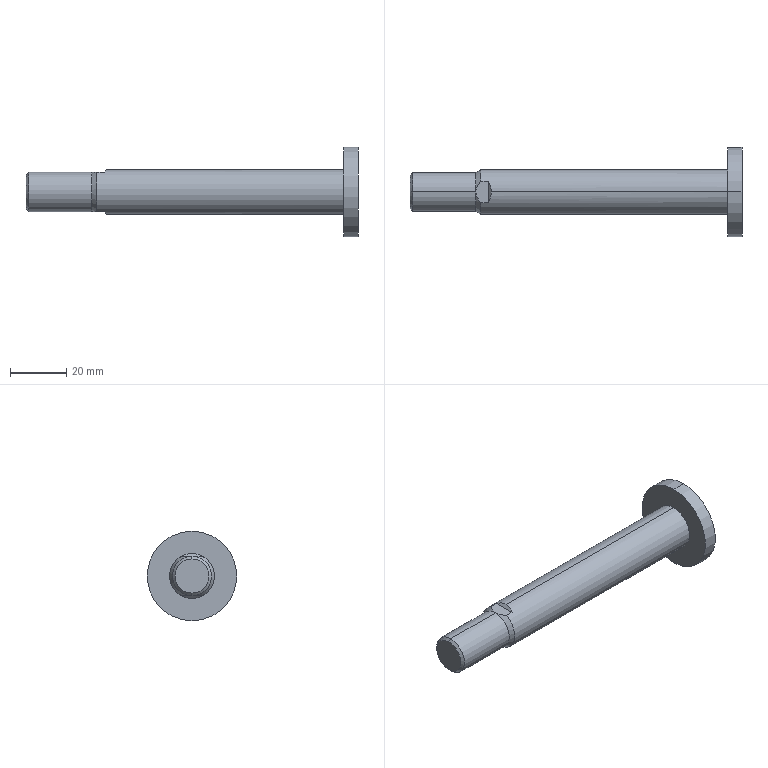Part | SolidWorks | features BaseBody 1 | 1 solid | 17 faces | box 118.5 x 32 x 32 mm | volume 25635 mm3 | plane 7 | cylinder 6 | cone 4 | commonest cylinder face diameters 14 x2 16 x2 32 x2
STEP:
#1=CARTESIAN_POINT('',(-0.5,3.873,7.));
#2=VERTEX_POINT('',#1);
#3=CARTESIAN_POINT('',(0.5,0.,8.));
#4=VERTEX_POINT('',#3);
#5=CARTESIAN_POINT('',(-0.5,3.873,7.));
#6=CARTESIAN_POINT('',(0.1595,2.681,7.659));
#7=CARTESIAN_POINT('',(0.5,1.362,8.));
#8=CARTESIAN_POINT('',(0.5,0.,8.));
#9=(BOUNDED_CURVE()B_SPLINE_CURVE(3,(#5,#6,#7,#8),.UNSPECIFIED.,.F.,.F.)B_SPLINE_CURVE_WITH_KNOTS((4,4),(5.778,6.283),.UNSPECIFIED.)CURVE()GEOMETRIC_REPRESENTATION_ITEM()RATIONAL_B_SPLINE_CURVE((1.,0.9788,0.9788,1.))REPRESENTATION_ITEM(''));
#10=EDGE_CURVE('',#2,#4,#9,.T.);
#11=ORIENTED_EDGE('',*,*,#10,.T.);
#12=CARTESIAN_POINT('',(85.,0.,8.));
#13=VERTEX_POINT('',#12);
#14=CARTESIAN_POINT('',(90.,0.,8.));
#15=DIRECTION('',(1.,0.,0.));
#16=VECTOR('',#15,1000.);
#17=LINE('',#14,#16);
#18=EDGE_CURVE('',#4,#13,#17,.T.);
#19=ORIENTED_EDGE('',*,*,#18,.T.);
#20=CARTESIAN_POINT('',(85.,0.,-8.));
#21=VERTEX_POINT('',#20);
#22=CARTESIAN_POINT('',(85.,0.,0.));
#23=DIRECTION('',(-1.,0.,0.));
#24=DIRECTION('',(0.,0.,-1.));
#25=AXIS2_PLACEMENT_3D('',#22,#23,#24);
#26=CIRCLE('',#25,8.);
#27=EDGE_CURVE('',#13,#21,#26,.T.);
#28=ORIENTED_EDGE('',*,*,#27,.T.);
#29=CARTESIAN_POINT('',(0.5,0.,-8.));
#30=VERTEX_POINT('',#29);
#31=CARTESIAN_POINT('',(90.,0.,-8.));
#32=DIRECTION('',(1.,0.,0.));
#33=VECTOR('',#32,1000.);
#34=LINE('',#31,#33);
#35=EDGE_CURVE('',#30,#21,#34,.T.);
#36=ORIENTED_EDGE('',*,*,#35,.F.);
#37=CARTESIAN_POINT('',(-0.5,3.873,-7.));
#38=VERTEX_POINT('',#37);
#39=CARTESIAN_POINT('',(0.5,0.,-8.));
#40=CARTESIAN_POINT('',(0.5,1.362,-8.));
#41=CARTESIAN_POINT('',(0.1595,2.681,-7.659));
#42=CARTESIAN_POINT('',(-0.5,3.873,-7.));
#43=(BOUNDED_CURVE()B_SPLINE_CURVE(3,(#39,#40,#41,#42),.UNSPECIFIED.,.F.,.F.)B_SPLINE_CURVE_WITH_KNOTS((4,4),(0.,0.5054),.UNSPECIFIED.)CURVE()GEOMETRIC_REPRESENTATION_ITEM()RATIONAL_B_SPLINE_CURVE((1.,0.9788,0.9788,1.))REPRESENTATION_ITEM(''));
#44=EDGE_CURVE('',#30,#38,#43,.T.);
#45=ORIENTED_EDGE('',*,*,#44,.T.);
#46=CARTESIAN_POINT('',(-3.268,3.873,-7.));
#47=VERTEX_POINT('',#46);
#48=CARTESIAN_POINT('',(90.,3.873,-7.));
#49=DIRECTION('',(-1.,0.,0.));
#50=VECTOR('',#49,1000.);
#51=LINE('',#48,#50);
#52=EDGE_CURVE('',#38,#47,#51,.T.);
#53=ORIENTED_EDGE('',*,*,#52,.T.);
#54=CARTESIAN_POINT('',(-3.268,3.873,7.));
#55=VERTEX_POINT('',#54);
#56=CARTESIAN_POINT('',(-3.268,0.,0.));
#57=DIRECTION('',(1.,0.,0.));
#58=DIRECTION('',(0.,0.,-1.));
#59=AXIS2_PLACEMENT_3D('',#56,#57,#58);
#60=CIRCLE('',#59,8.);
#61=EDGE_CURVE('',#47,#55,#60,.T.);
#62=ORIENTED_EDGE('',*,*,#61,.T.);
#63=CARTESIAN_POINT('',(90.,3.873,7.));
#64=DIRECTION('',(1.,0.,0.));
#65=VECTOR('',#64,1000.);
#66=LINE('',#63,#65);
#67=EDGE_CURVE('',#55,#2,#66,.T.);
#68=ORIENTED_EDGE('',*,*,#67,.T.);
#69=EDGE_LOOP('',(#11,#19,#28,#36,#45,#53,#62,#68));
#70=FACE_OUTER_BOUND('',#69,.T.);
#71=CARTESIAN_POINT('',(90.,0.,0.));
#72=DIRECTION('',(1.,0.,0.));
#73=DIRECTION('',(0.,0.,-1.));
#74=AXIS2_PLACEMENT_3D('',#71,#72,#73);
#75=CYLINDRICAL_SURFACE('',#74,8.);
#76=ADVANCED_FACE('',(#70),#75,.T.);
#77=CARTESIAN_POINT('',(-27.58,0.,-7.));
#78=VERTEX_POINT('',#77);
#79=CARTESIAN_POINT('',(-27.58,0.,7.));
#80=VERTEX_POINT('',#79);
#81=CARTESIAN_POINT('',(-27.58,0.,0.));
#82=DIRECTION('',(1.,0.,0.));
#83=DIRECTION('',(0.,0.,-1.));
#84=AXIS2_PLACEMENT_3D('',#81,#82,#83);
#85=CIRCLE('',#84,7.);
#86=EDGE_CURVE('',#78,#80,#85,.T.);
#87=ORIENTED_EDGE('',*,*,#86,.T.);
#88=CARTESIAN_POINT('',(-5.,0.,7.));
#89=VERTEX_POINT('',#88);
#90=CARTESIAN_POINT('',(90.,0.,7.));
#91=DIRECTION('',(1.,0.,0.));
#92=VECTOR('',#91,1000.);
#93=LINE('',#90,#92);
#94=EDGE_CURVE('',#80,#89,#93,.T.);
#95=ORIENTED_EDGE('',*,*,#94,.T.);
#96=CARTESIAN_POINT('',(-5.,0.,-7.));
#97=VERTEX_POINT('',#96);
#98=CARTESIAN_POINT('',(-5.,0.,0.));
#99=DIRECTION('',(1.,0.,0.));
#100=DIRECTION('',(0.,0.,-1.));
#101=AXIS2_PLACEMENT_3D('',#98,#99,#100);
#102=CIRCLE('',#101,7.);
#103=EDGE_CURVE('',#97,#89,#102,.T.);
#104=ORIENTED_EDGE('',*,*,#103,.F.);
#105=CARTESIAN_POINT('',(90.,0.,-7.));
#106=DIRECTION('',(1.,0.,0.));
#107=VECTOR('',#106,1000.);
#108=LINE('',#105,#107);
#109=EDGE_CURVE('',#78,#97,#108,.T.);
#110=ORIENTED_EDGE('',*,*,#109,.F.);
#111=EDGE_LOOP('',(#87,#95,#104,#110));
#112=FACE_OUTER_BOUND('',#111,.T.);
#113=CARTESIAN_POINT('',(90.,0.,0.));
#114=DIRECTION('',(1.,0.,0.));
#115=DIRECTION('',(0.,0.,-1.));
#116=AXIS2_PLACEMENT_3D('',#113,#114,#115);
#117=CYLINDRICAL_SURFACE('',#116,7.);
#118=ADVANCED_FACE('',(#112),#117,.T.);
#119=CARTESIAN_POINT('',(85.,0.,-16.));
#120=VERTEX_POINT('',#119);
#121=CARTESIAN_POINT('',(85.,0.,16.));
#122=VERTEX_POINT('',#121);
#123=CARTESIAN_POINT('',(85.,0.,0.));
#124=DIRECTION('',(1.,0.,0.));
#125=DIRECTION('',(0.,0.,-1.));
#126=AXIS2_PLACEMENT_3D('',#123,#124,#125);
#127=CIRCLE('',#126,16.);
#128=EDGE_CURVE('',#120,#122,#127,.T.);
#129=ORIENTED_EDGE('',*,*,#128,.T.);
#130=CARTESIAN_POINT('',(90.,0.,16.));
#131=VERTEX_POINT('',#130);
#132=CARTESIAN_POINT('',(90.,0.,16.));
#133=DIRECTION('',(1.,0.,0.));
#134=VECTOR('',#133,1000.);
#135=LINE('',#132,#134);
#136=EDGE_CURVE('',#122,#131,#135,.T.);
#137=ORIENTED_EDGE('',*,*,#136,.T.);
#138=CARTESIAN_POINT('',(90.,0.,-16.));
#139=VERTEX_POINT('',#138);
#140=CARTESIAN_POINT('',(90.,0.,0.));
#141=DIRECTION('',(-1.,0.,0.));
#142=DIRECTION('',(0.,0.,-1.));
#143=AXIS2_PLACEMENT_3D('',#140,#141,#142);
#144=CIRCLE('',#143,16.);
#145=EDGE_CURVE('',#131,#139,#144,.T.);
#146=ORIENTED_EDGE('',*,*,#145,.T.);
#147=CARTESIAN_POINT('',(90.,0.,-16.));
#148=DIRECTION('',(1.,0.,0.));
#149=VECTOR('',#148,1000.);
#150=LINE('',#147,#149);
#151=EDGE_CURVE('',#120,#139,#150,.T.);
#152=ORIENTED_EDGE('',*,*,#151,.F.);
#153=EDGE_LOOP('',(#129,#137,#146,#152));
#154=FACE_OUTER_BOUND('',#153,.T.);
#155=CARTESIAN_POINT('',(90.,0.,0.));
#156=DIRECTION('',(1.,0.,0.));
#157=DIRECTION('',(0.,0.,-1.));
#158=AXIS2_PLACEMENT_3D('',#155,#156,#157);
#159=CYLINDRICAL_SURFACE('',#158,16.);
#160=ADVANCED_FACE('',(#154),#159,.T.);
#161=CARTESIAN_POINT('',(-28.5,0.,-6.08));
#162=VERTEX_POINT('',#161);
#163=CARTESIAN_POINT('',(-28.5,0.,6.08));
#164=VERTEX_POINT('',#163);
#165=CARTESIAN_POINT('',(-28.5,0.,0.));
#166=DIRECTION('',(1.,0.,0.));
#167=DIRECTION('',(0.,0.,-1.));
#168=AXIS2_PLACEMENT_3D('',#165,#166,#167);
#169=CIRCLE('',#168,6.08);
#170=EDGE_CURVE('',#162,#164,#169,.T.);
#171=ORIENTED_EDGE('',*,*,#170,.T.);
#172=CARTESIAN_POINT('',(-27.58,0.,7.));
#173=DIRECTION('',(0.7071,0.,0.7071));
#174=VECTOR('',#173,1000.);
#175=LINE('',#172,#174);
#176=EDGE_CURVE('',#164,#80,#175,.T.);
#177=ORIENTED_EDGE('',*,*,#176,.T.);
#178=ORIENTED_EDGE('',*,*,#86,.F.);
#179=CARTESIAN_POINT('',(-27.58,0.,-7.));
#180=DIRECTION('',(0.7071,0.,-0.7071));
#181=VECTOR('',#180,1000.);
#182=LINE('',#179,#181);
#183=EDGE_CURVE('',#162,#78,#182,.T.);
#184=ORIENTED_EDGE('',*,*,#183,.F.);
#185=EDGE_LOOP('',(#171,#177,#178,#184));
#186=FACE_OUTER_BOUND('',#185,.T.);
#187=CARTESIAN_POINT('',(-27.58,0.,0.));
#188=DIRECTION('',(1.,0.,0.));
#189=DIRECTION('',(0.,0.,-1.));
#190=AXIS2_PLACEMENT_3D('',#187,#188,#189);
#191=CONICAL_SURFACE('',#190,7.,0.7854);
#192=ADVANCED_FACE('',(#186),#191,.T.);
#193=ORIENTED_EDGE('',*,*,#18,.F.);
#194=CARTESIAN_POINT('',(-0.5,-3.873,7.));
#195=VERTEX_POINT('',#194);
#196=CARTESIAN_POINT('',(0.5,0.,8.));
#197=CARTESIAN_POINT('',(0.5,-1.362,8.));
#198=CARTESIAN_POINT('',(0.1595,-2.681,7.659));
#199=CARTESIAN_POINT('',(-0.5,-3.873,7.));
#200=(BOUNDED_CURVE()B_SPLINE_CURVE(3,(#196,#197,#198,#199),.UNSPECIFIED.,.F.,.F.)B_SPLINE_CURVE_WITH_KNOTS((4,4),(0.,0.5054),.UNSPECIFIED.)CURVE()GEOMETRIC_REPRESENTATION_ITEM()RATIONAL_B_SPLINE_CURVE((1.,0.9788,0.9788,1.))REPRESENTATION_ITEM(''));
#201=EDGE_CURVE('',#4,#195,#200,.T.);
#202=ORIENTED_EDGE('',*,*,#201,.T.);
#203=CARTESIAN_POINT('',(-3.268,-3.873,7.));
#204=VERTEX_POINT('',#203);
#205=CARTESIAN_POINT('',(90.,-3.873,7.));
#206=DIRECTION('',(-1.,0.,0.));
#207=VECTOR('',#206,1000.);
#208=LINE('',#205,#207);
#209=EDGE_CURVE('',#195,#204,#208,.T.);
#210=ORIENTED_EDGE('',*,*,#209,.T.);
#211=CARTESIAN_POINT('',(-3.268,-3.873,-7.));
#212=VERTEX_POINT('',#211);
#213=CARTESIAN_POINT('',(-3.268,0.,0.));
#214=DIRECTION('',(1.,0.,0.));
#215=DIRECTION('',(0.,0.,-1.));
#216=AXIS2_PLACEMENT_3D('',#213,#214,#215);
#217=CIRCLE('',#216,8.);
#218=EDGE_CURVE('',#204,#212,#217,.T.);
#219=ORIENTED_EDGE('',*,*,#218,.T.);
#220=CARTESIAN_POINT('',(-0.5,-3.873,-7.));
#221=VERTEX_POINT('',#220);
#222=CARTESIAN_POINT('',(90.,-3.873,-7.));
#223=DIRECTION('',(1.,0.,0.));
#224=VECTOR('',#223,1000.);
#225=LINE('',#222,#224);
#226=EDGE_CURVE('',#212,#221,#225,.T.);
#227=ORIENTED_EDGE('',*,*,#226,.T.);
#228=CARTESIAN_POINT('',(-0.5,-3.873,-7.));
#229=CARTESIAN_POINT('',(0.1595,-2.681,-7.659));
#230=CARTESIAN_POINT('',(0.5,-1.362,-8.));
#231=CARTESIAN_POINT('',(0.5,0.,-8.));
#232=(BOUNDED_CURVE()B_SPLINE_CURVE(3,(#228,#229,#230,#231),.UNSPECIFIED.,.F.,.F.)B_SPLINE_CURVE_WITH_KNOTS((4,4),(5.778,6.283),.UNSPECIFIED.)CURVE()GEOMETRIC_REPRESENTATION_ITEM()RATIONAL_B_SPLINE_CURVE((1.,0.9788,0.9788,1.))REPRESENTATION_ITEM(''));
#233=EDGE_CURVE('',#221,#30,#232,.T.);
#234=ORIENTED_EDGE('',*,*,#233,.T.);
#235=ORIENTED_EDGE('',*,*,#35,.T.);
#236=CARTESIAN_POINT('',(85.,0.,0.));
#237=DIRECTION('',(-1.,0.,0.));
#238=DIRECTION('',(0.,0.,-1.));
#239=AXIS2_PLACEMENT_3D('',#236,#237,#238);
#240=CIRCLE('',#239,8.);
#241=EDGE_CURVE('',#21,#13,#240,.T.);
#242=ORIENTED_EDGE('',*,*,#241,.T.);
#243=EDGE_LOOP('',(#193,#202,#210,#219,#227,#234,#235,#242));
#244=FACE_OUTER_BOUND('',#243,.T.);
#245=CARTESIAN_POINT('',(90.,0.,0.));
#246=DIRECTION('',(1.,0.,0.));
#247=DIRECTION('',(0.,0.,-1.));
#248=AXIS2_PLACEMENT_3D('',#245,#246,#247);
#249=CYLINDRICAL_SURFACE('',#248,8.);
#250=ADVANCED_FACE('',(#244),#249,.T.);
#251=ORIENTED_EDGE('',*,*,#10,.F.);
#252=CARTESIAN_POINT('',(-0.5,16.,7.));
#253=DIRECTION('',(0.,-1.,0.));
#254=VECTOR('',#253,1000.);
#255=LINE('',#252,#254);
#256=EDGE_CURVE('',#2,#195,#255,.T.);
#257=ORIENTED_EDGE('',*,*,#256,.T.);
#258=ORIENTED_EDGE('',*,*,#201,.F.);
#259=EDGE_LOOP('',(#251,#257,#258));
#260=FACE_OUTER_BOUND('',#259,.T.);
#261=CARTESIAN_POINT('',(4.5,16.,12.));
#262=DIRECTION('',(-0.7071,0.,0.7071));
#263=DIRECTION('',(0.7071,0.,0.7071));
#264=AXIS2_PLACEMENT_3D('',#261,#262,#263);
#265=PLANE('',#264);
#266=ADVANCED_FACE('',(#260),#265,.T.);
#267=CARTESIAN_POINT('',(-3.268,3.873,7.));
#268=CARTESIAN_POINT('',(-3.734,3.318,7.));
#269=CARTESIAN_POINT('',(-4.153,2.734,7.));
#270=CARTESIAN_POINT('',(-4.632,1.764,7.));
#271=CARTESIAN_POINT('',(-4.767,1.421,7.));
#272=CARTESIAN_POINT('',(-4.95,0.7235,7.));
#273=CARTESIAN_POINT('',(-5.,0.3666,7.));
#274=CARTESIAN_POINT('',(-5.,0.,7.));
#275=B_SPLINE_CURVE_WITH_KNOTS('',3,(#267,#268,#269,#270,#271,#272,#273,#274),.UNSPECIFIED.,.F.,.F.,(4,2,2,4),(0.,0.002152,0.003229,0.004305),.UNSPECIFIED.);
#276=EDGE_CURVE('',#55,#89,#275,.T.);
#277=ORIENTED_EDGE('',*,*,#276,.T.);
#278=CARTESIAN_POINT('',(-5.,0.,7.));
#279=CARTESIAN_POINT('',(-5.,-0.3658,7.));
#280=CARTESIAN_POINT('',(-4.95,-0.7219,7.));
#281=CARTESIAN_POINT('',(-4.768,-1.418,7.));
#282=CARTESIAN_POINT('',(-4.634,-1.76,7.));
#283=CARTESIAN_POINT('',(-4.315,-2.407,7.));
#284=CARTESIAN_POINT('',(-4.129,-2.714,7.));
#285=CARTESIAN_POINT('',(-3.722,-3.308,7.));
#286=CARTESIAN_POINT('',(-3.501,-3.595,7.));
#287=CARTESIAN_POINT('',(-3.268,-3.873,7.));
#288=B_SPLINE_CURVE_WITH_KNOTS('',3,(#278,#279,#280,#281,#282,#283,#284,#285,#286,#287),.UNSPECIFIED.,.F.,.F.,(4,2,2,2,4),(0.,0.001077,0.002154,0.003231,0.004308),.UNSPECIFIED.);
#289=EDGE_CURVE('',#89,#204,#288,.T.);
#290=ORIENTED_EDGE('',*,*,#289,.T.);
#291=ORIENTED_EDGE('',*,*,#209,.F.);
#292=ORIENTED_EDGE('',*,*,#256,.F.);
#293=ORIENTED_EDGE('',*,*,#67,.F.);
#294=EDGE_LOOP('',(#277,#290,#291,#292,#293));
#295=FACE_OUTER_BOUND('',#294,.T.);
#296=CARTESIAN_POINT('',(-0.5,16.,7.));
#297=DIRECTION('',(0.,0.,1.));
#298=DIRECTION('',(1.,0.,0.));
#299=AXIS2_PLACEMENT_3D('',#296,#297,#298);
#300=PLANE('',#299);
#301=ADVANCED_FACE('',(#295),#300,.T.);
#302=CARTESIAN_POINT('',(-3.268,3.873,-7.));
#303=CARTESIAN_POINT('',(-3.734,3.318,-7.));
#304=CARTESIAN_POINT('',(-4.153,2.734,-7.));
#305=CARTESIAN_POINT('',(-4.632,1.764,-7.));
#306=CARTESIAN_POINT('',(-4.767,1.421,-7.));
#307=CARTESIAN_POINT('',(-4.95,0.7235,-7.));
#308=CARTESIAN_POINT('',(-5.,0.3666,-7.));
#309=CARTESIAN_POINT('',(-5.,0.,-7.));
#310=B_SPLINE_CURVE_WITH_KNOTS('',3,(#302,#303,#304,#305,#306,#307,#308,#309),.UNSPECIFIED.,.F.,.F.,(4,2,2,4),(0.,0.002152,0.003229,0.004305),.UNSPECIFIED.);
#311=EDGE_CURVE('',#47,#97,#310,.T.);
#312=ORIENTED_EDGE('',*,*,#311,.T.);
#313=ORIENTED_EDGE('',*,*,#103,.T.);
#314=ORIENTED_EDGE('',*,*,#276,.F.);
#315=ORIENTED_EDGE('',*,*,#61,.F.);
#316=EDGE_LOOP('',(#312,#313,#314,#315));
#317=FACE_OUTER_BOUND('',#316,.T.);
#318=CARTESIAN_POINT('',(-3.268,0.,0.));
#319=DIRECTION('',(1.,0.,0.));
#320=DIRECTION('',(0.,0.,-1.));
#321=AXIS2_PLACEMENT_3D('',#318,#319,#320);
#322=CONICAL_SURFACE('',#321,8.,0.5236);
#323=ADVANCED_FACE('',(#317),#322,.T.);
#324=CARTESIAN_POINT('',(-3.268,-3.873,-7.));
#325=CARTESIAN_POINT('',(-3.734,-3.318,-7.));
#326=CARTESIAN_POINT('',(-4.153,-2.734,-7.));
#327=CARTESIAN_POINT('',(-4.632,-1.764,-7.));
#328=CARTESIAN_POINT('',(-4.767,-1.421,-7.));
#329=CARTESIAN_POINT('',(-4.95,-0.7235,-7.));
#330=CARTESIAN_POINT('',(-5.,-0.3666,-7.));
#331=CARTESIAN_POINT('',(-5.,0.,-7.));
#332=B_SPLINE_CURVE_WITH_KNOTS('',3,(#324,#325,#326,#327,#328,#329,#330,#331),.UNSPECIFIED.,.F.,.F.,(4,2,2,4),(0.,0.002152,0.003229,0.004305),.UNSPECIFIED.);
#333=EDGE_CURVE('',#212,#97,#332,.T.);
#334=ORIENTED_EDGE('',*,*,#333,.T.);
#335=ORIENTED_EDGE('',*,*,#311,.F.);
#336=ORIENTED_EDGE('',*,*,#52,.F.);
#337=CARTESIAN_POINT('',(-0.5,16.,-7.));
#338=DIRECTION('',(0.,-1.,0.));
#339=VECTOR('',#338,1000.);
#340=LINE('',#337,#339);
#341=EDGE_CURVE('',#38,#221,#340,.T.);
#342=ORIENTED_EDGE('',*,*,#341,.T.);
#343=ORIENTED_EDGE('',*,*,#226,.F.);
#344=EDGE_LOOP('',(#334,#335,#336,#342,#343));
#345=FACE_OUTER_BOUND('',#344,.T.);
#346=CARTESIAN_POINT('',(-5.,16.,-7.));
#347=DIRECTION('',(0.,0.,-1.));
#348=DIRECTION('',(-1.,0.,0.));
#349=AXIS2_PLACEMENT_3D('',#346,#347,#348);
#350=PLANE('',#349);
#351=ADVANCED_FACE('',(#345),#350,.T.);
#352=ORIENTED_EDGE('',*,*,#233,.F.);
#353=ORIENTED_EDGE('',*,*,#341,.F.);
#354=ORIENTED_EDGE('',*,*,#44,.F.);
#355=EDGE_LOOP('',(#352,#353,#354));
#356=FACE_OUTER_BOUND('',#355,.T.);
#357=CARTESIAN_POINT('',(-0.5,16.,-7.));
#358=DIRECTION('',(-0.7071,0.,-0.7071));
#359=DIRECTION('',(-0.7071,0.,0.7071));
#360=AXIS2_PLACEMENT_3D('',#357,#358,#359);
#361=PLANE('',#360);
#362=ADVANCED_FACE('',(#356),#361,.T.);
#363=ORIENTED_EDGE('',*,*,#333,.F.);
#364=ORIENTED_EDGE('',*,*,#218,.F.);
#365=ORIENTED_EDGE('',*,*,#289,.F.);
#366=CARTESIAN_POINT('',(-5.,0.,0.));
#367=DIRECTION('',(1.,0.,0.));
#368=DIRECTION('',(0.,0.,-1.));
#369=AXIS2_PLACEMENT_3D('',#366,#367,#368);
#370=CIRCLE('',#369,7.);
#371=EDGE_CURVE('',#89,#97,#370,.T.);
#372=ORIENTED_EDGE('',*,*,#371,.T.);
#373=EDGE_LOOP('',(#363,#364,#365,#372));
#374=FACE_OUTER_BOUND('',#373,.T.);
#375=CARTESIAN_POINT('',(-3.268,0.,0.));
#376=DIRECTION('',(1.,0.,0.));
#377=DIRECTION('',(0.,0.,-1.));
#378=AXIS2_PLACEMENT_3D('',#375,#376,#377);
#379=CONICAL_SURFACE('',#378,8.,0.5236);
#380=ADVANCED_FACE('',(#374),#379,.T.);
#381=ORIENTED_EDGE('',*,*,#241,.F.);
#382=ORIENTED_EDGE('',*,*,#27,.F.);
#383=EDGE_LOOP('',(#381,#382));
#384=FACE_BOUND('',#383,.T.);
#385=ORIENTED_EDGE('',*,*,#128,.F.);
#386=CARTESIAN_POINT('',(85.,0.,0.));
#387=DIRECTION('',(1.,0.,0.));
#388=DIRECTION('',(0.,0.,-1.));
#389=AXIS2_PLACEMENT_3D('',#386,#387,#388);
#390=CIRCLE('',#389,16.);
#391=EDGE_CURVE('',#122,#120,#390,.T.);
#392=ORIENTED_EDGE('',*,*,#391,.F.);
#393=EDGE_LOOP('',(#385,#392));
#394=FACE_OUTER_BOUND('',#393,.T.);
#395=CARTESIAN_POINT('',(85.,8.,0.));
#396=DIRECTION('',(1.,0.,0.));
#397=DIRECTION('',(0.,0.,-1.));
#398=AXIS2_PLACEMENT_3D('',#395,#396,#397);
#399=PLANE('',#398);
#400=ADVANCED_FACE('',(#384,#394),#399,.F.);
#401=ORIENTED_EDGE('',*,*,#94,.F.);
#402=CARTESIAN_POINT('',(-27.58,0.,0.));
#403=DIRECTION('',(1.,0.,0.));
#404=DIRECTION('',(0.,0.,-1.));
#405=AXIS2_PLACEMENT_3D('',#402,#403,#404);
#406=CIRCLE('',#405,7.);
#407=EDGE_CURVE('',#80,#78,#406,.T.);
#408=ORIENTED_EDGE('',*,*,#407,.T.);
#409=ORIENTED_EDGE('',*,*,#109,.T.);
#410=ORIENTED_EDGE('',*,*,#371,.F.);
#411=EDGE_LOOP('',(#401,#408,#409,#410));
#412=FACE_OUTER_BOUND('',#411,.T.);
#413=CARTESIAN_POINT('',(90.,0.,0.));
#414=DIRECTION('',(1.,0.,0.));
#415=DIRECTION('',(0.,0.,-1.));
#416=AXIS2_PLACEMENT_3D('',#413,#414,#415);
#417=CYLINDRICAL_SURFACE('',#416,7.);
#418=ADVANCED_FACE('',(#412),#417,.T.);
#419=ORIENTED_EDGE('',*,*,#136,.F.);
#420=ORIENTED_EDGE('',*,*,#391,.T.);
#421=ORIENTED_EDGE('',*,*,#151,.T.);
#422=CARTESIAN_POINT('',(90.,0.,0.));
#423=DIRECTION('',(-1.,0.,0.));
#424=DIRECTION('',(0.,0.,-1.));
#425=AXIS2_PLACEMENT_3D('',#422,#423,#424);
#426=CIRCLE('',#425,16.);
#427=EDGE_CURVE('',#139,#131,#426,.T.);
#428=ORIENTED_EDGE('',*,*,#427,.T.);
#429=EDGE_LOOP('',(#419,#420,#421,#428));
#430=FACE_OUTER_BOUND('',#429,.T.);
#431=CARTESIAN_POINT('',(90.,0.,0.));
#432=DIRECTION('',(1.,0.,0.));
#433=DIRECTION('',(0.,0.,-1.));
#434=AXIS2_PLACEMENT_3D('',#431,#432,#433);
#435=CYLINDRICAL_SURFACE('',#434,16.);
#436=ADVANCED_FACE('',(#430),#435,.T.);
#437=ORIENTED_EDGE('',*,*,#176,.F.);
#438=CARTESIAN_POINT('',(-28.5,0.,0.));
#439=DIRECTION('',(1.,0.,0.));
#440=DIRECTION('',(0.,0.,-1.));
#441=AXIS2_PLACEMENT_3D('',#438,#439,#440);
#442=CIRCLE('',#441,6.08);
#443=EDGE_CURVE('',#164,#162,#442,.T.);
#444=ORIENTED_EDGE('',*,*,#443,.T.);
#445=ORIENTED_EDGE('',*,*,#183,.T.);
#446=ORIENTED_EDGE('',*,*,#407,.F.);
#447=EDGE_LOOP('',(#437,#444,#445,#446));
#448=FACE_OUTER_BOUND('',#447,.T.);
#449=CARTESIAN_POINT('',(-27.58,0.,0.));
#450=DIRECTION('',(1.,0.,0.));
#451=DIRECTION('',(0.,0.,-1.));
#452=AXIS2_PLACEMENT_3D('',#449,#450,#451);
#453=CONICAL_SURFACE('',#452,7.,0.7854);
#454=ADVANCED_FACE('',(#448),#453,.T.);
#455=ORIENTED_EDGE('',*,*,#427,.F.);
#456=ORIENTED_EDGE('',*,*,#145,.F.);
#457=EDGE_LOOP('',(#455,#456));
#458=FACE_OUTER_BOUND('',#457,.T.);
#459=CARTESIAN_POINT('',(90.,16.,0.));
#460=DIRECTION('',(-1.,0.,0.));
#461=DIRECTION('',(0.,0.,1.));
#462=AXIS2_PLACEMENT_3D('',#459,#460,#461);
#463=PLANE('',#462);
#464=ADVANCED_FACE('',(#458),#463,.F.);
#465=ORIENTED_EDGE('',*,*,#170,.F.);
#466=ORIENTED_EDGE('',*,*,#443,.F.);
#467=EDGE_LOOP('',(#465,#466));
#468=FACE_OUTER_BOUND('',#467,.T.);
#469=CARTESIAN_POINT('',(-28.5,0.,0.));
#470=DIRECTION('',(1.,0.,0.));
#471=DIRECTION('',(0.,0.,-1.));
#472=AXIS2_PLACEMENT_3D('',#469,#470,#471);
#473=PLANE('',#472);
#474=ADVANCED_FACE('',(#468),#473,.F.);
#475=CLOSED_SHELL('',(#76,#118,#160,#192,#250,#266,#301,#323,#351,#362,#380,#400,#418,#436,#454,#464,#474));
#476=MANIFOLD_SOLID_BREP('',#475);
#477=CARTESIAN_POINT('',(0.,0.,0.));
#478=DIRECTION('',(0.,0.,1.));
#479=DIRECTION('',(1.,0.,0.));
#480=AXIS2_PLACEMENT_3D('',#477,#478,#479);
#481=(LENGTH_UNIT()NAMED_UNIT(*)SI_UNIT(.MILLI.,.METRE.));
#482=UNCERTAINTY_MEASURE_WITH_UNIT(LENGTH_MEASURE(0.00001),#481,'','');
#483=(NAMED_UNIT(*)PLANE_ANGLE_UNIT()SI_UNIT($,.RADIAN.));
#484=(NAMED_UNIT(*)SI_UNIT($,.STERADIAN.)SOLID_ANGLE_UNIT());
#485=(GEOMETRIC_REPRESENTATION_CONTEXT(3)GLOBAL_UNCERTAINTY_ASSIGNED_CONTEXT((#482))GLOBAL_UNIT_ASSIGNED_CONTEXT((#481,#483,#484))REPRESENTATION_CONTEXT('',''));
#486=ADVANCED_BREP_SHAPE_REPRESENTATION('',(#476,#480),#485);